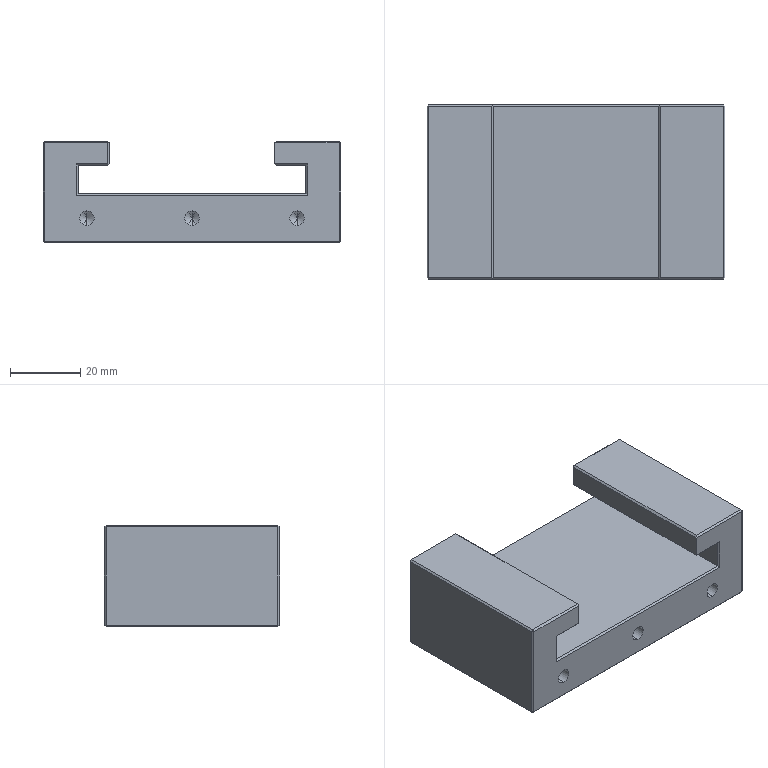Part | SolidWorks | features Chamfer 2, Extrusion 1, HoleWzd 1, ICE 1, MoveFace 1 | 1 solid | 68 faces | box 85 x 50 x 29 mm | volume 80145 mm3 | plane 56 | cylinder 6 | cone 6 | commonest cylinder face diameters 4.2 x6